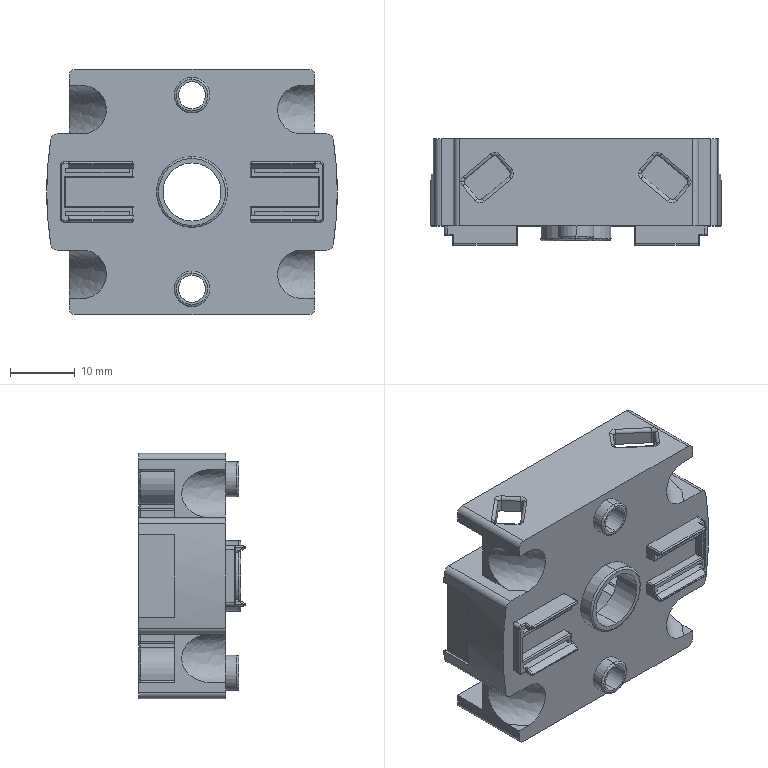Part | STEP file | PCS-11A-3_1_2.stp | 1 solid | 548 faces | box 45 x 16.5 x 38 mm | volume 7553 mm3 | plane 257 | cylinder 209 | torus 55 | sphere 23 | spline 4 | commonest cylinder face diameters 0.6 x62 0.4 x59 1 x45 2 x8 6 x6 4.2 x4